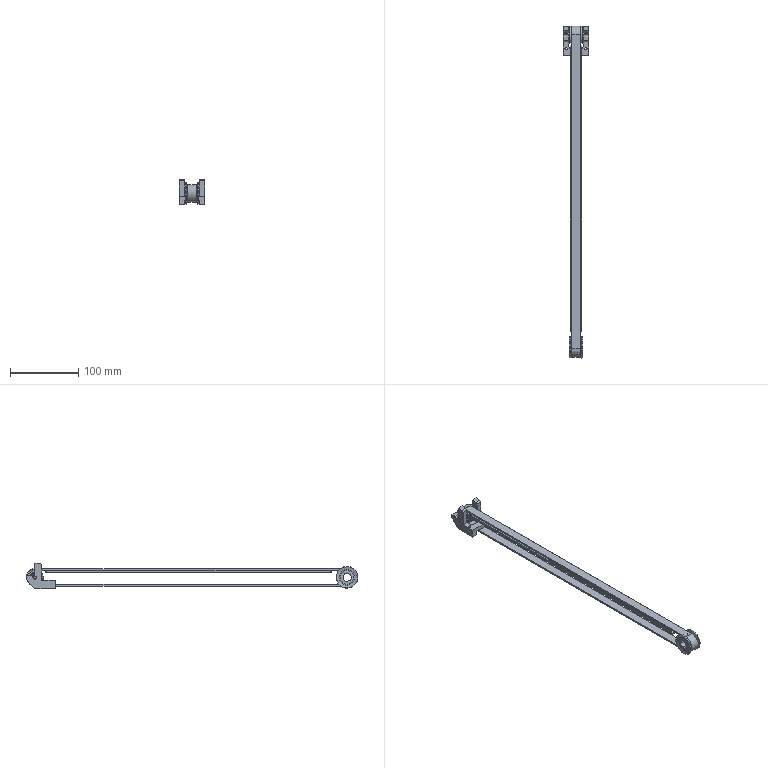Part | NX | features BREP 12 | 13 solids | 712 faces | box 37 x 486.5 x 37 mm | volume 83530 mm3 | cylinder 345 | plane 269 | cone 62 | torus 36 | commonest cylinder face diameters 1.22 x152 20.95 x34 23.75 x30 3.4 x12 5 x10 3.242 x8